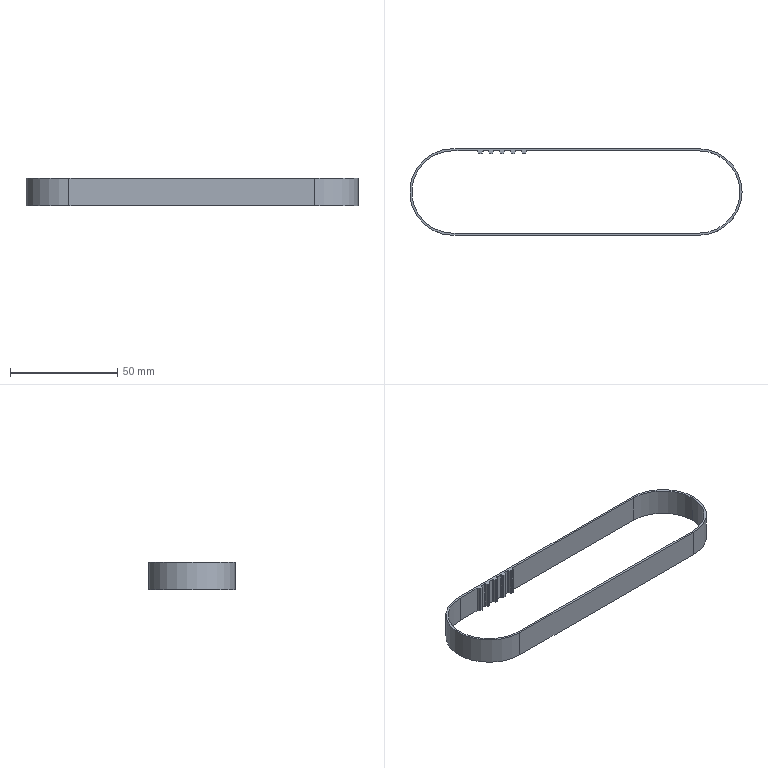Part | STEP file | TBN138XL050_info-1-24-24 | 1 solid | 52 faces | box 154.6 x 40.3 x 12.7 mm | volume 4631 mm3 | cylinder 26 | plane 26 | commonest cylinder face diameters 0.76 x20 38.3 x3 40.3 x3